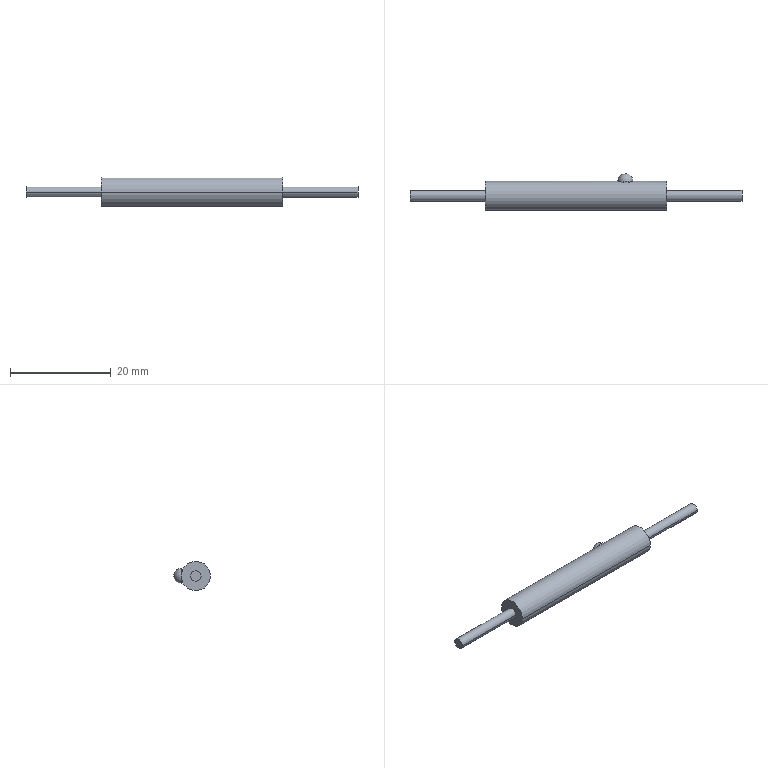Part | NX | 1 solid | 13 faces | box 66 x 7.3 x 5.8 mm | volume 1063 mm3 | cylinder 6 | plane 4 | sphere 3 | commonest cylinder face diameters 2.1 x4 5.8 x2
STEP:
#1=CARTESIAN_POINT('',(0.,-2.9,0.));
#2=VERTEX_POINT('',#1);
#3=CARTESIAN_POINT('',(0.,2.9,0.));
#4=VERTEX_POINT('',#3);
#5=CARTESIAN_POINT('',(0.,0.,0.));
#6=DIRECTION('',(1.,0.,0.));
#7=DIRECTION('',(0.,1.,0.));
#8=AXIS2_PLACEMENT_3D('',#5,#6,#7);
#9=CIRCLE('',#8,2.9);
#10=EDGE_CURVE('',#2,#4,#9,.T.);
#11=ORIENTED_EDGE('',*,*,#10,.F.);
#12=CARTESIAN_POINT('',(0.,0.,0.));
#13=DIRECTION('',(1.,0.,0.));
#14=DIRECTION('',(0.,1.,0.));
#15=AXIS2_PLACEMENT_3D('',#12,#13,#14);
#16=CIRCLE('',#15,2.9);
#17=EDGE_CURVE('',#4,#2,#16,.T.);
#18=ORIENTED_EDGE('',*,*,#17,.F.);
#19=EDGE_LOOP('',(#11,#18));
#20=FACE_BOUND('',#19,.T.);
#21=CARTESIAN_POINT('',(0.,1.05,0.));
#22=VERTEX_POINT('',#21);
#23=CARTESIAN_POINT('',(0.,-1.05,0.));
#24=VERTEX_POINT('',#23);
#25=CARTESIAN_POINT('',(0.,0.,0.));
#26=DIRECTION('',(-1.,0.,0.));
#27=DIRECTION('',(0.,-1.,0.));
#28=AXIS2_PLACEMENT_3D('',#25,#26,#27);
#29=CIRCLE('',#28,1.05);
#30=EDGE_CURVE('',#22,#24,#29,.T.);
#31=ORIENTED_EDGE('',*,*,#30,.F.);
#32=CARTESIAN_POINT('',(0.,0.,0.));
#33=DIRECTION('',(-1.,0.,0.));
#34=DIRECTION('',(0.,-1.,0.));
#35=AXIS2_PLACEMENT_3D('',#32,#33,#34);
#36=CIRCLE('',#35,1.05);
#37=EDGE_CURVE('',#24,#22,#36,.T.);
#38=ORIENTED_EDGE('',*,*,#37,.F.);
#39=EDGE_LOOP('',(#31,#38));
#40=FACE_BOUND('',#39,.T.);
#41=CARTESIAN_POINT('',(0.,0.,0.));
#42=DIRECTION('',(1.,0.,0.));
#43=DIRECTION('',(0.,1.,0.));
#44=AXIS2_PLACEMENT_3D('',#41,#42,#43);
#45=PLANE('',#44);
#46=ADVANCED_FACE('',(#20,#40),#45,.F.);
#47=CARTESIAN_POINT('',(36.,-2.9,0.));
#48=VERTEX_POINT('',#47);
#49=CARTESIAN_POINT('',(36.,2.9,0.));
#50=VERTEX_POINT('',#49);
#51=CARTESIAN_POINT('',(36.,0.,0.));
#52=DIRECTION('',(-1.,0.,0.));
#53=DIRECTION('',(0.,-1.,0.));
#54=AXIS2_PLACEMENT_3D('',#51,#52,#53);
#55=CIRCLE('',#54,2.9);
#56=EDGE_CURVE('',#48,#50,#55,.T.);
#57=ORIENTED_EDGE('',*,*,#56,.T.);
#58=CARTESIAN_POINT('',(29.3,2.9,0.));
#59=VERTEX_POINT('',#58);
#60=CARTESIAN_POINT('',(0.,2.9,0.));
#61=DIRECTION('',(1.,0.,0.));
#62=VECTOR('',#61,1000.);
#63=LINE('',#60,#62);
#64=EDGE_CURVE('',#59,#50,#63,.T.);
#65=ORIENTED_EDGE('',*,*,#64,.F.);
#66=CARTESIAN_POINT('',(26.3,2.9,0.));
#67=VERTEX_POINT('',#66);
#68=CARTESIAN_POINT('',(29.3,2.9,0.));
#69=CARTESIAN_POINT('',(29.3,2.9,0.3886));
#70=CARTESIAN_POINT('',(28.988,2.71,1.156));
#71=CARTESIAN_POINT('',(27.783,2.41,1.602));
#72=CARTESIAN_POINT('',(26.592,2.721,1.13));
#73=CARTESIAN_POINT('',(26.3,2.9,0.3815));
#74=CARTESIAN_POINT('',(26.3,2.9,0.));
#75=B_SPLINE_CURVE_WITH_KNOTS('',3,(#68,#69,#70,#71,#72,#73,#74),.UNSPECIFIED.,.F.,.F.,(4,1,1,1,4),(0.,0.25,0.5,0.75,1.),.UNSPECIFIED.);
#76=EDGE_CURVE('',#67,#59,#75,.F.);
#77=ORIENTED_EDGE('',*,*,#76,.F.);
#78=CARTESIAN_POINT('',(0.,2.9,0.));
#79=DIRECTION('',(1.,0.,0.));
#80=VECTOR('',#79,1000.);
#81=LINE('',#78,#80);
#82=EDGE_CURVE('',#4,#67,#81,.T.);
#83=ORIENTED_EDGE('',*,*,#82,.F.);
#84=ORIENTED_EDGE('',*,*,#17,.T.);
#85=CARTESIAN_POINT('',(0.,-2.9,0.));
#86=DIRECTION('',(1.,0.,0.));
#87=VECTOR('',#86,1000.);
#88=LINE('',#85,#87);
#89=EDGE_CURVE('',#2,#48,#88,.T.);
#90=ORIENTED_EDGE('',*,*,#89,.T.);
#91=EDGE_LOOP('',(#57,#65,#77,#83,#84,#90));
#92=FACE_BOUND('',#91,.T.);
#93=CARTESIAN_POINT('',(0.,0.,0.));
#94=DIRECTION('',(1.,0.,0.));
#95=DIRECTION('',(0.,-1.,0.));
#96=AXIS2_PLACEMENT_3D('',#93,#94,#95);
#97=CYLINDRICAL_SURFACE('',#96,2.9);
#98=ADVANCED_FACE('',(#92),#97,.T.);
#99=CARTESIAN_POINT('',(51.,-1.05,0.));
#100=VERTEX_POINT('',#99);
#101=CARTESIAN_POINT('',(51.,1.05,0.));
#102=VERTEX_POINT('',#101);
#103=CARTESIAN_POINT('',(51.,0.,0.));
#104=DIRECTION('',(-1.,0.,0.));
#105=DIRECTION('',(0.,-1.,0.));
#106=AXIS2_PLACEMENT_3D('',#103,#104,#105);
#107=CIRCLE('',#106,1.05);
#108=EDGE_CURVE('',#100,#102,#107,.T.);
#109=ORIENTED_EDGE('',*,*,#108,.F.);
#110=CARTESIAN_POINT('',(51.,0.,0.));
#111=DIRECTION('',(-1.,0.,0.));
#112=DIRECTION('',(0.,-1.,0.));
#113=AXIS2_PLACEMENT_3D('',#110,#111,#112);
#114=CIRCLE('',#113,1.05);
#115=EDGE_CURVE('',#102,#100,#114,.T.);
#116=ORIENTED_EDGE('',*,*,#115,.F.);
#117=EDGE_LOOP('',(#109,#116));
#118=FACE_BOUND('',#117,.T.);
#119=CARTESIAN_POINT('',(51.,0.,0.));
#120=DIRECTION('',(1.,0.,0.));
#121=DIRECTION('',(0.,1.,0.));
#122=AXIS2_PLACEMENT_3D('',#119,#120,#121);
#123=PLANE('',#122);
#124=ADVANCED_FACE('',(#118),#123,.T.);
#125=CARTESIAN_POINT('',(27.8,2.9,0.));
#126=DIRECTION('',(0.,1.,0.));
#127=DIRECTION('',(1.,0.,0.));
#128=AXIS2_PLACEMENT_3D('',#125,#126,#127);
#129=CIRCLE('',#128,1.5);
#130=EDGE_CURVE('',#59,#67,#129,.T.);
#131=ORIENTED_EDGE('',*,*,#130,.F.);
#132=CARTESIAN_POINT('',(26.3,2.9,0.));
#133=CARTESIAN_POINT('',(26.3,2.9,-0.3884));
#134=CARTESIAN_POINT('',(26.611,2.71,-1.155));
#135=CARTESIAN_POINT('',(27.817,2.41,-1.602));
#136=CARTESIAN_POINT('',(29.008,2.721,-1.13));
#137=CARTESIAN_POINT('',(29.3,2.9,-0.3816));
#138=CARTESIAN_POINT('',(29.3,2.9,0.));
#139=B_SPLINE_CURVE_WITH_KNOTS('',3,(#132,#133,#134,#135,#136,#137,#138),.UNSPECIFIED.,.F.,.F.,(4,1,1,1,4),(0.,0.25,0.5,0.75,1.),.UNSPECIFIED.);
#140=EDGE_CURVE('',#59,#67,#139,.F.);
#141=ORIENTED_EDGE('',*,*,#140,.T.);
#142=EDGE_LOOP('',(#131,#141));
#143=FACE_BOUND('',#142,.T.);
#144=CARTESIAN_POINT('',(27.8,2.9,0.));
#145=DIRECTION('',(0.,1.,0.));
#146=DIRECTION('',(1.,0.,0.));
#147=AXIS2_PLACEMENT_3D('',#144,#145,#146);
#148=SPHERICAL_SURFACE('',#147,1.5);
#149=ADVANCED_FACE('',(#143),#148,.T.);
#150=CARTESIAN_POINT('',(-15.,-1.05,0.));
#151=VERTEX_POINT('',#150);
#152=CARTESIAN_POINT('',(-15.,1.05,0.));
#153=VERTEX_POINT('',#152);
#154=CARTESIAN_POINT('',(-15.,0.,0.));
#155=DIRECTION('',(1.,0.,0.));
#156=DIRECTION('',(0.,-1.,0.));
#157=AXIS2_PLACEMENT_3D('',#154,#155,#156);
#158=CIRCLE('',#157,1.05);
#159=EDGE_CURVE('',#151,#153,#158,.T.);
#160=ORIENTED_EDGE('',*,*,#159,.T.);
#161=CARTESIAN_POINT('',(0.,1.05,0.));
#162=DIRECTION('',(-1.,0.,0.));
#163=VECTOR('',#162,1000.);
#164=LINE('',#161,#163);
#165=EDGE_CURVE('',#22,#153,#164,.T.);
#166=ORIENTED_EDGE('',*,*,#165,.F.);
#167=ORIENTED_EDGE('',*,*,#30,.T.);
#168=CARTESIAN_POINT('',(0.,-1.05,0.));
#169=DIRECTION('',(-1.,0.,0.));
#170=VECTOR('',#169,1000.);
#171=LINE('',#168,#170);
#172=EDGE_CURVE('',#24,#151,#171,.T.);
#173=ORIENTED_EDGE('',*,*,#172,.T.);
#174=EDGE_LOOP('',(#160,#166,#167,#173));
#175=FACE_BOUND('',#174,.T.);
#176=CARTESIAN_POINT('',(0.,0.,0.));
#177=DIRECTION('',(-1.,0.,0.));
#178=DIRECTION('',(0.,1.,0.));
#179=AXIS2_PLACEMENT_3D('',#176,#177,#178);
#180=CYLINDRICAL_SURFACE('',#179,1.05);
#181=ADVANCED_FACE('',(#175),#180,.T.);
#182=ORIENTED_EDGE('',*,*,#56,.F.);
#183=CARTESIAN_POINT('',(36.,0.,0.));
#184=DIRECTION('',(-1.,0.,0.));
#185=DIRECTION('',(0.,-1.,0.));
#186=AXIS2_PLACEMENT_3D('',#183,#184,#185);
#187=CIRCLE('',#186,2.9);
#188=EDGE_CURVE('',#50,#48,#187,.T.);
#189=ORIENTED_EDGE('',*,*,#188,.F.);
#190=EDGE_LOOP('',(#182,#189));
#191=FACE_BOUND('',#190,.T.);
#192=CARTESIAN_POINT('',(36.,-1.05,0.));
#193=VERTEX_POINT('',#192);
#194=CARTESIAN_POINT('',(36.,1.05,0.));
#195=VERTEX_POINT('',#194);
#196=CARTESIAN_POINT('',(36.,0.,0.));
#197=DIRECTION('',(1.,0.,0.));
#198=DIRECTION('',(0.,1.,0.));
#199=AXIS2_PLACEMENT_3D('',#196,#197,#198);
#200=CIRCLE('',#199,1.05);
#201=EDGE_CURVE('',#193,#195,#200,.T.);
#202=ORIENTED_EDGE('',*,*,#201,.F.);
#203=CARTESIAN_POINT('',(36.,0.,0.));
#204=DIRECTION('',(1.,0.,0.));
#205=DIRECTION('',(0.,1.,0.));
#206=AXIS2_PLACEMENT_3D('',#203,#204,#205);
#207=CIRCLE('',#206,1.05);
#208=EDGE_CURVE('',#195,#193,#207,.T.);
#209=ORIENTED_EDGE('',*,*,#208,.F.);
#210=EDGE_LOOP('',(#202,#209));
#211=FACE_BOUND('',#210,.T.);
#212=CARTESIAN_POINT('',(36.,0.,0.));
#213=DIRECTION('',(1.,0.,0.));
#214=DIRECTION('',(0.,1.,0.));
#215=AXIS2_PLACEMENT_3D('',#212,#213,#214);
#216=PLANE('',#215);
#217=ADVANCED_FACE('',(#191,#211),#216,.T.);
#218=ORIENTED_EDGE('',*,*,#108,.T.);
#219=CARTESIAN_POINT('',(36.,1.05,0.));
#220=DIRECTION('',(1.,0.,0.));
#221=VECTOR('',#220,1000.);
#222=LINE('',#219,#221);
#223=EDGE_CURVE('',#195,#102,#222,.T.);
#224=ORIENTED_EDGE('',*,*,#223,.F.);
#225=ORIENTED_EDGE('',*,*,#208,.T.);
#226=CARTESIAN_POINT('',(36.,-1.05,0.));
#227=DIRECTION('',(1.,0.,0.));
#228=VECTOR('',#227,1000.);
#229=LINE('',#226,#228);
#230=EDGE_CURVE('',#193,#100,#229,.T.);
#231=ORIENTED_EDGE('',*,*,#230,.T.);
#232=EDGE_LOOP('',(#218,#224,#225,#231));
#233=FACE_BOUND('',#232,.T.);
#234=CARTESIAN_POINT('',(36.,0.,0.));
#235=DIRECTION('',(1.,0.,0.));
#236=DIRECTION('',(0.,-1.,0.));
#237=AXIS2_PLACEMENT_3D('',#234,#235,#236);
#238=CYLINDRICAL_SURFACE('',#237,1.05);
#239=ADVANCED_FACE('',(#233),#238,.T.);
#240=ORIENTED_EDGE('',*,*,#159,.F.);
#241=CARTESIAN_POINT('',(-15.,0.,0.));
#242=DIRECTION('',(1.,0.,0.));
#243=DIRECTION('',(0.,-1.,0.));
#244=AXIS2_PLACEMENT_3D('',#241,#242,#243);
#245=CIRCLE('',#244,1.05);
#246=EDGE_CURVE('',#153,#151,#245,.T.);
#247=ORIENTED_EDGE('',*,*,#246,.F.);
#248=EDGE_LOOP('',(#240,#247));
#249=FACE_BOUND('',#248,.T.);
#250=CARTESIAN_POINT('',(-15.,0.,0.));
#251=DIRECTION('',(-1.,0.,0.));
#252=DIRECTION('',(0.,0.,1.));
#253=AXIS2_PLACEMENT_3D('',#250,#251,#252);
#254=PLANE('',#253);
#255=ADVANCED_FACE('',(#249),#254,.T.);
#256=ORIENTED_EDGE('',*,*,#201,.T.);
#257=ORIENTED_EDGE('',*,*,#223,.T.);
#258=ORIENTED_EDGE('',*,*,#115,.T.);
#259=ORIENTED_EDGE('',*,*,#230,.F.);
#260=EDGE_LOOP('',(#256,#257,#258,#259));
#261=FACE_BOUND('',#260,.T.);
#262=CARTESIAN_POINT('',(36.,0.,0.));
#263=DIRECTION('',(1.,0.,0.));
#264=DIRECTION('',(0.,-1.,0.));
#265=AXIS2_PLACEMENT_3D('',#262,#263,#264);
#266=CYLINDRICAL_SURFACE('',#265,1.05);
#267=ADVANCED_FACE('',(#261),#266,.T.);
#268=ORIENTED_EDGE('',*,*,#10,.T.);
#269=ORIENTED_EDGE('',*,*,#82,.T.);
#270=ORIENTED_EDGE('',*,*,#140,.F.);
#271=ORIENTED_EDGE('',*,*,#64,.T.);
#272=ORIENTED_EDGE('',*,*,#188,.T.);
#273=ORIENTED_EDGE('',*,*,#89,.F.);
#274=EDGE_LOOP('',(#268,#269,#270,#271,#272,#273));
#275=FACE_BOUND('',#274,.T.);
#276=CARTESIAN_POINT('',(0.,0.,0.));
#277=DIRECTION('',(1.,0.,0.));
#278=DIRECTION('',(0.,-1.,0.));
#279=AXIS2_PLACEMENT_3D('',#276,#277,#278);
#280=CYLINDRICAL_SURFACE('',#279,2.9);
#281=ADVANCED_FACE('',(#275),#280,.T.);
#282=ORIENTED_EDGE('',*,*,#165,.T.);
#283=ORIENTED_EDGE('',*,*,#246,.T.);
#284=ORIENTED_EDGE('',*,*,#172,.F.);
#285=ORIENTED_EDGE('',*,*,#37,.T.);
#286=EDGE_LOOP('',(#282,#283,#284,#285));
#287=FACE_BOUND('',#286,.T.);
#288=CARTESIAN_POINT('',(0.,0.,0.));
#289=DIRECTION('',(-1.,0.,0.));
#290=DIRECTION('',(0.,1.,0.));
#291=AXIS2_PLACEMENT_3D('',#288,#289,#290);
#292=CYLINDRICAL_SURFACE('',#291,1.05);
#293=ADVANCED_FACE('',(#287),#292,.T.);
#294=ORIENTED_EDGE('',*,*,#130,.T.);
#295=CARTESIAN_POINT('',(27.8,2.9,1.5));
#296=VERTEX_POINT('',#295);
#297=CARTESIAN_POINT('',(27.8,2.9,0.));
#298=DIRECTION('',(0.,1.,0.));
#299=DIRECTION('',(1.,0.,0.));
#300=AXIS2_PLACEMENT_3D('',#297,#298,#299);
#301=CIRCLE('',#300,1.5);
#302=EDGE_CURVE('',#67,#296,#301,.T.);
#303=ORIENTED_EDGE('',*,*,#302,.T.);
#304=CARTESIAN_POINT('',(27.8,2.9,0.));
#305=DIRECTION('',(0.,1.,0.));
#306=DIRECTION('',(1.,0.,0.));
#307=AXIS2_PLACEMENT_3D('',#304,#305,#306);
#308=CIRCLE('',#307,1.5);
#309=EDGE_CURVE('',#296,#59,#308,.T.);
#310=ORIENTED_EDGE('',*,*,#309,.T.);
#311=EDGE_LOOP('',(#294,#303,#310));
#312=FACE_BOUND('',#311,.T.);
#313=CARTESIAN_POINT('',(27.8,2.9,0.));
#314=DIRECTION('',(0.,1.,0.));
#315=DIRECTION('',(1.,0.,0.));
#316=AXIS2_PLACEMENT_3D('',#313,#314,#315);
#317=SPHERICAL_SURFACE('',#316,1.5);
#318=ADVANCED_FACE('',(#312),#317,.T.);
#319=ORIENTED_EDGE('',*,*,#302,.F.);
#320=ORIENTED_EDGE('',*,*,#76,.T.);
#321=ORIENTED_EDGE('',*,*,#309,.F.);
#322=EDGE_LOOP('',(#319,#320,#321));
#323=FACE_BOUND('',#322,.T.);
#324=CARTESIAN_POINT('',(27.8,2.9,0.));
#325=DIRECTION('',(0.,1.,0.));
#326=DIRECTION('',(1.,0.,0.));
#327=AXIS2_PLACEMENT_3D('',#324,#325,#326);
#328=SPHERICAL_SURFACE('',#327,1.5);
#329=ADVANCED_FACE('',(#323),#328,.T.);
#330=CLOSED_SHELL('',(#46,#98,#124,#149,#181,#217,#239,#255,#267,#281,#293,#318,#329));
#331=MANIFOLD_SOLID_BREP('',#330);
#332=(LENGTH_UNIT()NAMED_UNIT(*)SI_UNIT(.MILLI.,.METRE.));
#333=UNCERTAINTY_MEASURE_WITH_UNIT(LENGTH_MEASURE(0.0508),#332,'','');
#334=(NAMED_UNIT(*)PLANE_ANGLE_UNIT()SI_UNIT($,.RADIAN.));
#335=(NAMED_UNIT(*)SI_UNIT($,.STERADIAN.)SOLID_ANGLE_UNIT());
#336=(GEOMETRIC_REPRESENTATION_CONTEXT(3)GLOBAL_UNCERTAINTY_ASSIGNED_CONTEXT((#333))GLOBAL_UNIT_ASSIGNED_CONTEXT((#332,#334,#335))REPRESENTATION_CONTEXT('',''));
#337=ADVANCED_BREP_SHAPE_REPRESENTATION('',(#331),#336);